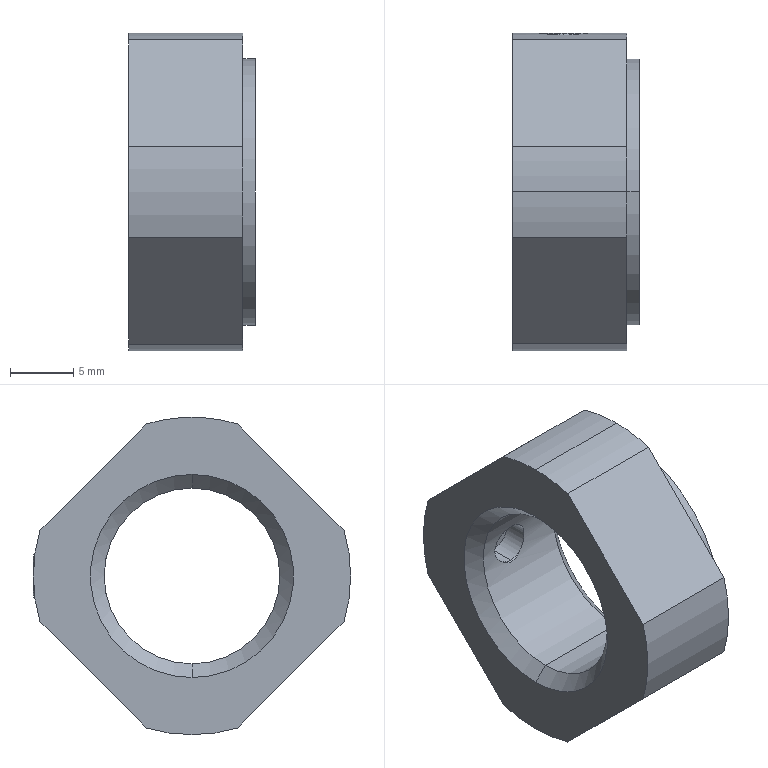Part | STEP file | BNG16 | 2 solids | 48 faces | box 10 x 25 x 25 mm | volume 2769 mm3 | cone 19 | plane 16 | cylinder 13 | commonest cylinder face diameters 25 x5 3.242 x2 4 x2 13.835 x2 21 x2
STEP:
#1=CARTESIAN_POINT('',(8.918,0.,-6.918));
#2=VERTEX_POINT('',#1);
#3=CARTESIAN_POINT('',(8.918,0.,6.918));
#4=VERTEX_POINT('',#3);
#5=CARTESIAN_POINT('',(8.918,0.,0.));
#6=DIRECTION('',(-1.,0.,0.));
#7=DIRECTION('',(0.,0.,1.));
#8=AXIS2_PLACEMENT_3D('',#5,#6,#7);
#9=CIRCLE('',#8,6.918);
#10=EDGE_CURVE('',#2,#4,#9,.T.);
#11=ORIENTED_EDGE('',*,*,#10,.F.);
#12=CARTESIAN_POINT('',(1.083,0.,-6.918));
#13=VERTEX_POINT('',#12);
#14=CARTESIAN_POINT('',(10.,0.,-6.918));
#15=DIRECTION('',(-1.,0.,0.));
#16=VECTOR('',#15,1000.);
#17=LINE('',#14,#16);
#18=EDGE_CURVE('',#2,#13,#17,.T.);
#19=ORIENTED_EDGE('',*,*,#18,.T.);
#20=CARTESIAN_POINT('',(1.083,0.,6.918));
#21=VERTEX_POINT('',#20);
#22=CARTESIAN_POINT('',(1.083,0.,0.));
#23=DIRECTION('',(1.,0.,0.));
#24=DIRECTION('',(0.,0.,1.));
#25=AXIS2_PLACEMENT_3D('',#22,#23,#24);
#26=CIRCLE('',#25,6.918);
#27=EDGE_CURVE('',#21,#13,#26,.T.);
#28=ORIENTED_EDGE('',*,*,#27,.F.);
#29=CARTESIAN_POINT('',(10.,0.,6.918));
#30=DIRECTION('',(-1.,0.,0.));
#31=VECTOR('',#30,1000.);
#32=LINE('',#29,#31);
#33=EDGE_CURVE('',#4,#21,#32,.T.);
#34=ORIENTED_EDGE('',*,*,#33,.F.);
#35=EDGE_LOOP('',(#11,#19,#28,#34));
#36=FACE_OUTER_BOUND('',#35,.T.);
#37=CARTESIAN_POINT('',(10.,0.,0.));
#38=DIRECTION('',(-1.,0.,0.));
#39=DIRECTION('',(0.,0.,1.));
#40=AXIS2_PLACEMENT_3D('',#37,#38,#39);
#41=CYLINDRICAL_SURFACE('',#40,6.918);
#42=ADVANCED_FACE('',(#36),#41,.F.);
#43=ORIENTED_EDGE('',*,*,#27,.T.);
#44=CARTESIAN_POINT('',(0.,0.,-8.));
#45=VERTEX_POINT('',#44);
#46=CARTESIAN_POINT('',(0.,0.,-8.));
#47=DIRECTION('',(-0.7071,0.,-0.7071));
#48=VECTOR('',#47,1000.);
#49=LINE('',#46,#48);
#50=EDGE_CURVE('',#13,#45,#49,.T.);
#51=ORIENTED_EDGE('',*,*,#50,.T.);
#52=CARTESIAN_POINT('',(0.,0.,8.));
#53=VERTEX_POINT('',#52);
#54=CARTESIAN_POINT('',(0.,0.,0.));
#55=DIRECTION('',(1.,0.,0.));
#56=DIRECTION('',(0.,0.,1.));
#57=AXIS2_PLACEMENT_3D('',#54,#55,#56);
#58=CIRCLE('',#57,8.);
#59=EDGE_CURVE('',#53,#45,#58,.T.);
#60=ORIENTED_EDGE('',*,*,#59,.F.);
#61=CARTESIAN_POINT('',(0.,0.,8.));
#62=DIRECTION('',(-0.7071,0.,0.7071));
#63=VECTOR('',#62,1000.);
#64=LINE('',#61,#63);
#65=EDGE_CURVE('',#21,#53,#64,.T.);
#66=ORIENTED_EDGE('',*,*,#65,.F.);
#67=EDGE_LOOP('',(#43,#51,#60,#66));
#68=FACE_OUTER_BOUND('',#67,.T.);
#69=CARTESIAN_POINT('',(0.,0.,0.));
#70=DIRECTION('',(-1.,0.,0.));
#71=DIRECTION('',(0.,0.,1.));
#72=AXIS2_PLACEMENT_3D('',#69,#70,#71);
#73=CONICAL_SURFACE('',#72,8.,0.7854);
#74=ADVANCED_FACE('',(#68),#73,.F.);
#75=CARTESIAN_POINT('',(4.,6.797,-1.621));
#76=VERTEX_POINT('',#75);
#77=CARTESIAN_POINT('',(3.016,6.796,-1.288));
#78=VERTEX_POINT('',#77);
#79=CARTESIAN_POINT('',(4.,6.797,0.));
#80=DIRECTION('',(0.,1.,0.));
#81=DIRECTION('',(0.,0.,1.));
#82=AXIS2_PLACEMENT_3D('',#79,#80,#81);
#83=CIRCLE('',#82,1.621);
#84=EDGE_CURVE('',#76,#78,#83,.T.);
#85=ORIENTED_EDGE('',*,*,#84,.F.);
#86=CARTESIAN_POINT('',(4.,12.121,-1.621));
#87=VERTEX_POINT('',#86);
#88=CARTESIAN_POINT('',(4.,6.418,-1.621));
#89=DIRECTION('',(0.,1.,0.));
#90=VECTOR('',#89,1000.);
#91=LINE('',#88,#90);
#92=EDGE_CURVE('',#76,#87,#91,.T.);
#93=ORIENTED_EDGE('',*,*,#92,.T.);
#94=CARTESIAN_POINT('',(4.,12.121,1.621));
#95=VERTEX_POINT('',#94);
#96=CARTESIAN_POINT('',(4.,12.121,0.));
#97=DIRECTION('',(0.,-1.,0.));
#98=DIRECTION('',(0.,0.,1.));
#99=AXIS2_PLACEMENT_3D('',#96,#97,#98);
#100=CIRCLE('',#99,1.621);
#101=EDGE_CURVE('',#95,#87,#100,.T.);
#102=ORIENTED_EDGE('',*,*,#101,.F.);
#103=CARTESIAN_POINT('',(4.,6.797,1.621));
#104=VERTEX_POINT('',#103);
#105=CARTESIAN_POINT('',(4.,6.418,1.621));
#106=DIRECTION('',(0.,1.,0.));
#107=VECTOR('',#106,1000.);
#108=LINE('',#105,#107);
#109=EDGE_CURVE('',#104,#95,#108,.T.);
#110=ORIENTED_EDGE('',*,*,#109,.F.);
#111=CARTESIAN_POINT('',(3.016,6.797,1.288));
#112=VERTEX_POINT('',#111);
#113=CARTESIAN_POINT('',(4.,6.797,0.));
#114=DIRECTION('',(0.,1.,0.));
#115=DIRECTION('',(0.,0.,1.));
#116=AXIS2_PLACEMENT_3D('',#113,#114,#115);
#117=CIRCLE('',#116,1.621);
#118=EDGE_CURVE('',#112,#104,#117,.T.);
#119=ORIENTED_EDGE('',*,*,#118,.F.);
#120=CARTESIAN_POINT('',(3.016,6.797,1.288));
#121=CARTESIAN_POINT('',(2.917,6.811,1.212));
#122=CARTESIAN_POINT('',(2.828,6.826,1.127));
#123=CARTESIAN_POINT('',(2.671,6.854,0.9367));
#124=CARTESIAN_POINT('',(2.603,6.868,0.8309));
#125=CARTESIAN_POINT('',(2.438,6.903,0.4991));
#126=CARTESIAN_POINT('',(2.379,6.917,0.2501));
#127=CARTESIAN_POINT('',(2.379,6.918,-0.1225));
#128=CARTESIAN_POINT('',(2.393,6.914,-0.2484));
#129=CARTESIAN_POINT('',(2.45,6.901,-0.4896));
#130=CARTESIAN_POINT('',(2.492,6.892,-0.6074));
#131=CARTESIAN_POINT('',(2.602,6.868,-0.8305));
#132=CARTESIAN_POINT('',(2.669,6.855,-0.934));
#133=CARTESIAN_POINT('',(2.827,6.826,-1.125));
#134=CARTESIAN_POINT('',(2.917,6.811,-1.212));
#135=CARTESIAN_POINT('',(3.016,6.796,-1.288));
#136=B_SPLINE_CURVE_WITH_KNOTS('',3,(#120,#121,#122,#123,#124,#125,#126,#127,#128,#129,#130,#131,#132,#133,#134,#135),.UNSPECIFIED.,.F.,.F.,(4,2,2,2,2,2,2,4),(0.,0.0003717,0.0007433,0.001487,0.001858,0.00223,0.002602,0.002973),.UNSPECIFIED.);
#137=EDGE_CURVE('',#112,#78,#136,.T.);
#138=ORIENTED_EDGE('',*,*,#137,.T.);
#139=EDGE_LOOP('',(#85,#93,#102,#110,#119,#138));
#140=FACE_OUTER_BOUND('',#139,.T.);
#141=CARTESIAN_POINT('',(4.,6.418,0.));
#142=DIRECTION('',(0.,1.,0.));
#143=DIRECTION('',(0.,0.,1.));
#144=AXIS2_PLACEMENT_3D('',#141,#142,#143);
#145=CYLINDRICAL_SURFACE('',#144,1.621);
#146=ADVANCED_FACE('',(#140),#145,.F.);
#147=ORIENTED_EDGE('',*,*,#10,.T.);
#148=CARTESIAN_POINT('',(10.,0.,8.));
#149=VERTEX_POINT('',#148);
#150=CARTESIAN_POINT('',(10.,0.,8.));
#151=DIRECTION('',(0.7071,0.,0.7071));
#152=VECTOR('',#151,1000.);
#153=LINE('',#150,#152);
#154=EDGE_CURVE('',#4,#149,#153,.T.);
#155=ORIENTED_EDGE('',*,*,#154,.T.);
#156=CARTESIAN_POINT('',(10.,0.,-8.));
#157=VERTEX_POINT('',#156);
#158=CARTESIAN_POINT('',(10.,0.,0.));
#159=DIRECTION('',(-1.,0.,0.));
#160=DIRECTION('',(0.,0.,-1.));
#161=AXIS2_PLACEMENT_3D('',#158,#159,#160);
#162=CIRCLE('',#161,8.);
#163=EDGE_CURVE('',#157,#149,#162,.T.);
#164=ORIENTED_EDGE('',*,*,#163,.F.);
#165=CARTESIAN_POINT('',(10.,0.,-8.));
#166=DIRECTION('',(0.7071,0.,-0.7071));
#167=VECTOR('',#166,1000.);
#168=LINE('',#165,#167);
#169=EDGE_CURVE('',#2,#157,#168,.T.);
#170=ORIENTED_EDGE('',*,*,#169,.F.);
#171=EDGE_LOOP('',(#147,#155,#164,#170));
#172=FACE_OUTER_BOUND('',#171,.T.);
#173=CARTESIAN_POINT('',(10.,0.,0.));
#174=DIRECTION('',(1.,0.,0.));
#175=DIRECTION('',(0.,0.,-1.));
#176=AXIS2_PLACEMENT_3D('',#173,#174,#175);
#177=CONICAL_SURFACE('',#176,8.,0.7854);
#178=ADVANCED_FACE('',(#172),#177,.F.);
#179=ORIENTED_EDGE('',*,*,#101,.T.);
#180=CARTESIAN_POINT('',(4.,12.361,-1.861));
#181=VERTEX_POINT('',#180);
#182=CARTESIAN_POINT('',(4.,12.504,-2.004));
#183=DIRECTION('',(0.,0.7071,-0.7071));
#184=VECTOR('',#183,1000.);
#185=LINE('',#182,#184);
#186=EDGE_CURVE('',#87,#181,#185,.T.);
#187=ORIENTED_EDGE('',*,*,#186,.T.);
#188=CARTESIAN_POINT('',(4.,12.361,1.861));
#189=VERTEX_POINT('',#188);
#190=CARTESIAN_POINT('',(4.,12.361,1.861));
#191=CARTESIAN_POINT('',(3.748,12.361,1.861));
#192=CARTESIAN_POINT('',(3.493,12.368,1.815));
#193=CARTESIAN_POINT('',(3.022,12.392,1.64));
#194=CARTESIAN_POINT('',(2.8,12.41,1.507));
#195=CARTESIAN_POINT('',(2.427,12.446,1.172));
#196=CARTESIAN_POINT('',(2.271,12.465,0.9655));
#197=CARTESIAN_POINT('',(2.058,12.492,0.51));
#198=CARTESIAN_POINT('',(2.,12.5,0.2533));
#199=CARTESIAN_POINT('',(2.,12.5,-0.1267));
#200=CARTESIAN_POINT('',(2.014,12.498,-0.2518));
#201=CARTESIAN_POINT('',(2.069,12.491,-0.4988));
#202=CARTESIAN_POINT('',(2.11,12.485,-0.6203));
#203=CARTESIAN_POINT('',(2.269,12.465,-0.9631));
#204=CARTESIAN_POINT('',(2.424,12.446,-1.17));
#205=CARTESIAN_POINT('',(2.706,12.419,-1.423));
#206=CARTESIAN_POINT('',(2.809,12.41,-1.498));
#207=CARTESIAN_POINT('',(3.025,12.394,-1.628));
#208=CARTESIAN_POINT('',(3.138,12.386,-1.683));
#209=CARTESIAN_POINT('',(3.495,12.368,-1.816));
#210=CARTESIAN_POINT('',(3.745,12.361,-1.861));
#211=CARTESIAN_POINT('',(4.,12.361,-1.861));
#212=B_SPLINE_CURVE_WITH_KNOTS('',3,(#190,#191,#192,#193,#194,#195,#196,#197,#198,#199,#200,#201,#202,#203,#204,#205,#206,#207,#208,#209,#210,#211),.UNSPECIFIED.,.F.,.F.,(4,2,2,2,2,2,2,2,2,2,4),(0.009167,0.009923,0.01068,0.01143,0.01219,0.01257,0.01294,0.0137,0.01408,0.01445,0.01521),.UNSPECIFIED.);
#213=EDGE_CURVE('',#189,#181,#212,.T.);
#214=ORIENTED_EDGE('',*,*,#213,.F.);
#215=CARTESIAN_POINT('',(4.,12.504,2.004));
#216=DIRECTION('',(0.,0.7071,0.7071));
#217=VECTOR('',#216,1000.);
#218=LINE('',#215,#217);
#219=EDGE_CURVE('',#95,#189,#218,.T.);
#220=ORIENTED_EDGE('',*,*,#219,.F.);
#221=EDGE_LOOP('',(#179,#187,#214,#220));
#222=FACE_OUTER_BOUND('',#221,.T.);
#223=CARTESIAN_POINT('',(4.,12.504,0.));
#224=DIRECTION('',(0.,1.,0.));
#225=DIRECTION('',(0.,0.,1.));
#226=AXIS2_PLACEMENT_3D('',#223,#224,#225);
#227=CONICAL_SURFACE('',#226,2.004,0.7854);
#228=ADVANCED_FACE('',(#222),#227,.F.);
#229=CARTESIAN_POINT('',(9.,-3.58,11.976));
#230=VERTEX_POINT('',#229);
#231=CARTESIAN_POINT('',(9.,0.,12.5));
#232=VERTEX_POINT('',#231);
#233=CARTESIAN_POINT('',(9.,0.,0.));
#234=DIRECTION('',(-1.,0.,0.));
#235=DIRECTION('',(0.,0.,1.));
#236=AXIS2_PLACEMENT_3D('',#233,#234,#235);
#237=CIRCLE('',#236,12.5);
#238=EDGE_CURVE('',#230,#232,#237,.T.);
#239=ORIENTED_EDGE('',*,*,#238,.T.);
#240=CARTESIAN_POINT('',(0.,0.,12.5));
#241=VERTEX_POINT('',#240);
#242=CARTESIAN_POINT('',(10.,0.,12.5));
#243=DIRECTION('',(-1.,0.,0.));
#244=VECTOR('',#243,1000.);
#245=LINE('',#242,#244);
#246=EDGE_CURVE('',#232,#241,#245,.T.);
#247=ORIENTED_EDGE('',*,*,#246,.T.);
#248=CARTESIAN_POINT('',(0.,-3.58,11.976));
#249=VERTEX_POINT('',#248);
#250=CARTESIAN_POINT('',(0.,0.,0.));
#251=DIRECTION('',(-1.,0.,0.));
#252=DIRECTION('',(0.,0.,1.));
#253=AXIS2_PLACEMENT_3D('',#250,#251,#252);
#254=CIRCLE('',#253,12.5);
#255=EDGE_CURVE('',#249,#241,#254,.T.);
#256=ORIENTED_EDGE('',*,*,#255,.F.);
#257=CARTESIAN_POINT('',(10.,-3.58,11.976));
#258=DIRECTION('',(1.,0.,0.));
#259=VECTOR('',#258,1000.);
#260=LINE('',#257,#259);
#261=EDGE_CURVE('',#249,#230,#260,.T.);
#262=ORIENTED_EDGE('',*,*,#261,.T.);
#263=EDGE_LOOP('',(#239,#247,#256,#262));
#264=FACE_OUTER_BOUND('',#263,.T.);
#265=CARTESIAN_POINT('',(10.,0.,0.));
#266=DIRECTION('',(-1.,0.,0.));
#267=DIRECTION('',(0.,0.,1.));
#268=AXIS2_PLACEMENT_3D('',#265,#266,#267);
#269=CYLINDRICAL_SURFACE('',#268,12.5);
#270=ADVANCED_FACE('',(#264),#269,.T.);
#271=CARTESIAN_POINT('',(10.,0.,-10.5));
#272=VERTEX_POINT('',#271);
#273=CARTESIAN_POINT('',(10.,0.,10.5));
#274=VERTEX_POINT('',#273);
#275=CARTESIAN_POINT('',(10.,0.,0.));
#276=DIRECTION('',(1.,0.,0.));
#277=DIRECTION('',(0.,0.,1.));
#278=AXIS2_PLACEMENT_3D('',#275,#276,#277);
#279=CIRCLE('',#278,10.5);
#280=EDGE_CURVE('',#272,#274,#279,.T.);
#281=ORIENTED_EDGE('',*,*,#280,.F.);
#282=CARTESIAN_POINT('',(9.,0.,-10.5));
#283=VERTEX_POINT('',#282);
#284=CARTESIAN_POINT('',(10.,0.,-10.5));
#285=DIRECTION('',(-1.,0.,0.));
#286=VECTOR('',#285,1000.);
#287=LINE('',#284,#286);
#288=EDGE_CURVE('',#272,#283,#287,.T.);
#289=ORIENTED_EDGE('',*,*,#288,.T.);
#290=CARTESIAN_POINT('',(9.,0.,10.5));
#291=VERTEX_POINT('',#290);
#292=CARTESIAN_POINT('',(9.,0.,0.));
#293=DIRECTION('',(1.,0.,0.));
#294=DIRECTION('',(0.,0.,1.));
#295=AXIS2_PLACEMENT_3D('',#292,#293,#294);
#296=CIRCLE('',#295,10.5);
#297=EDGE_CURVE('',#283,#291,#296,.T.);
#298=ORIENTED_EDGE('',*,*,#297,.T.);
#299=CARTESIAN_POINT('',(10.,0.,10.5));
#300=DIRECTION('',(-1.,0.,0.));
#301=VECTOR('',#300,1000.);
#302=LINE('',#299,#301);
#303=EDGE_CURVE('',#274,#291,#302,.T.);
#304=ORIENTED_EDGE('',*,*,#303,.F.);
#305=EDGE_LOOP('',(#281,#289,#298,#304));
#306=FACE_OUTER_BOUND('',#305,.T.);
#307=CARTESIAN_POINT('',(10.,0.,0.));
#308=DIRECTION('',(-1.,0.,0.));
#309=DIRECTION('',(0.,0.,1.));
#310=AXIS2_PLACEMENT_3D('',#307,#308,#309);
#311=CYLINDRICAL_SURFACE('',#310,10.5);
#312=ADVANCED_FACE('',(#306),#311,.T.);
#313=ORIENTED_EDGE('',*,*,#18,.F.);
#314=CARTESIAN_POINT('',(8.918,0.,0.));
#315=DIRECTION('',(-1.,0.,0.));
#316=DIRECTION('',(0.,0.,1.));
#317=AXIS2_PLACEMENT_3D('',#314,#315,#316);
#318=CIRCLE('',#317,6.918);
#319=EDGE_CURVE('',#4,#2,#318,.T.);
#320=ORIENTED_EDGE('',*,*,#319,.F.);
#321=ORIENTED_EDGE('',*,*,#33,.T.);
#322=CARTESIAN_POINT('',(1.083,0.,0.));
#323=DIRECTION('',(1.,0.,0.));
#324=DIRECTION('',(0.,0.,1.));
#325=AXIS2_PLACEMENT_3D('',#322,#323,#324);
#326=CIRCLE('',#325,6.918);
#327=EDGE_CURVE('',#13,#21,#326,.T.);
#328=ORIENTED_EDGE('',*,*,#327,.F.);
#329=EDGE_LOOP('',(#313,#320,#321,#328));
#330=FACE_OUTER_BOUND('',#329,.T.);
#331=CARTESIAN_POINT('',(4.984,6.796,1.288));
#332=VERTEX_POINT('',#331);
#333=CARTESIAN_POINT('',(4.984,6.796,1.288));
#334=CARTESIAN_POINT('',(4.919,6.784,1.353));
#335=CARTESIAN_POINT('',(4.849,6.772,1.412));
#336=CARTESIAN_POINT('',(4.7,6.749,1.517));
#337=CARTESIAN_POINT('',(4.62,6.739,1.563));
#338=CARTESIAN_POINT('',(4.452,6.721,1.638));
#339=CARTESIAN_POINT('',(4.366,6.714,1.667));
#340=CARTESIAN_POINT('',(4.187,6.704,1.706));
#341=CARTESIAN_POINT('',(4.094,6.701,1.716));
#342=CARTESIAN_POINT('',(3.817,6.701,1.717));
#343=CARTESIAN_POINT('',(3.633,6.712,1.676));
#344=CARTESIAN_POINT('',(3.299,6.747,1.527));
#345=CARTESIAN_POINT('',(3.146,6.772,1.419));
#346=CARTESIAN_POINT('',(3.016,6.797,1.288));
#347=B_SPLINE_CURVE_WITH_KNOTS('',3,(#333,#334,#335,#336,#337,#338,#339,#340,#341,#342,#343,#344,#345,#346),.UNSPECIFIED.,.F.,.F.,(4,2,2,2,2,2,4),(0.,0.0002754,0.0005508,0.0008262,0.001102,0.001652,0.002203),.UNSPECIFIED.);
#348=EDGE_CURVE('',#332,#112,#347,.T.);
#349=ORIENTED_EDGE('',*,*,#348,.F.);
#350=CARTESIAN_POINT('',(4.984,6.797,-1.288));
#351=VERTEX_POINT('',#350);
#352=CARTESIAN_POINT('',(4.984,6.797,-1.288));
#353=CARTESIAN_POINT('',(5.083,6.811,-1.212));
#354=CARTESIAN_POINT('',(5.172,6.826,-1.127));
#355=CARTESIAN_POINT('',(5.329,6.854,-0.9367));
#356=CARTESIAN_POINT('',(5.397,6.868,-0.8309));
#357=CARTESIAN_POINT('',(5.562,6.903,-0.4991));
#358=CARTESIAN_POINT('',(5.621,6.917,-0.2501));
#359=CARTESIAN_POINT('',(5.621,6.918,0.1225));
#360=CARTESIAN_POINT('',(5.607,6.914,0.2484));
#361=CARTESIAN_POINT('',(5.55,6.901,0.4896));
#362=CARTESIAN_POINT('',(5.508,6.892,0.6074));
#363=CARTESIAN_POINT('',(5.398,6.868,0.8305));
#364=CARTESIAN_POINT('',(5.331,6.855,0.934));
#365=CARTESIAN_POINT('',(5.173,6.826,1.125));
#366=CARTESIAN_POINT('',(5.083,6.811,1.212));
#367=CARTESIAN_POINT('',(4.984,6.796,1.288));
#368=B_SPLINE_CURVE_WITH_KNOTS('',3,(#352,#353,#354,#355,#356,#357,#358,#359,#360,#361,#362,#363,#364,#365,#366,#367),.UNSPECIFIED.,.F.,.F.,(4,2,2,2,2,2,2,4),(0.,0.0003717,0.0007433,0.001487,0.001858,0.00223,0.002602,0.002973),.UNSPECIFIED.);
#369=EDGE_CURVE('',#351,#332,#368,.T.);
#370=ORIENTED_EDGE('',*,*,#369,.F.);
#371=CARTESIAN_POINT('',(3.016,6.796,-1.288));
#372=CARTESIAN_POINT('',(3.081,6.784,-1.353));
#373=CARTESIAN_POINT('',(3.151,6.772,-1.412));
#374=CARTESIAN_POINT('',(3.3,6.749,-1.517));
#375=CARTESIAN_POINT('',(3.38,6.739,-1.563));
#376=CARTESIAN_POINT('',(3.548,6.721,-1.638));
#377=CARTESIAN_POINT('',(3.634,6.714,-1.667));
#378=CARTESIAN_POINT('',(3.813,6.704,-1.706));
#379=CARTESIAN_POINT('',(3.906,6.701,-1.716));
#380=CARTESIAN_POINT('',(4.183,6.701,-1.717));
#381=CARTESIAN_POINT('',(4.367,6.712,-1.676));
#382=CARTESIAN_POINT('',(4.701,6.747,-1.527));
#383=CARTESIAN_POINT('',(4.854,6.772,-1.419));
#384=CARTESIAN_POINT('',(4.984,6.797,-1.288));
#385=B_SPLINE_CURVE_WITH_KNOTS('',3,(#371,#372,#373,#374,#375,#376,#377,#378,#379,#380,#381,#382,#383,#384),.UNSPECIFIED.,.F.,.F.,(4,2,2,2,2,2,4),(0.,0.0002754,0.0005508,0.0008262,0.001102,0.001652,0.002203),.UNSPECIFIED.);
#386=EDGE_CURVE('',#78,#351,#385,.T.);
#387=ORIENTED_EDGE('',*,*,#386,.F.);
#388=ORIENTED_EDGE('',*,*,#137,.F.);
#389=EDGE_LOOP('',(#349,#370,#387,#388));
#390=FACE_BOUND('',#389,.T.);
#391=CARTESIAN_POINT('',(10.,0.,0.));
#392=DIRECTION('',(-1.,0.,0.));
#393=DIRECTION('',(0.,0.,1.));
#394=AXIS2_PLACEMENT_3D('',#391,#392,#393);
#395=CYLINDRICAL_SURFACE('',#394,6.918);
#396=ADVANCED_FACE('',(#330,#390),#395,.F.);
#397=ORIENTED_EDGE('',*,*,#50,.F.);
#398=ORIENTED_EDGE('',*,*,#327,.T.);
#399=ORIENTED_EDGE('',*,*,#65,.T.);
#400=CARTESIAN_POINT('',(0.,0.,0.));
#401=DIRECTION('',(1.,0.,0.));
#402=DIRECTION('',(0.,0.,1.));
#403=AXIS2_PLACEMENT_3D('',#400,#401,#402);
#404=CIRCLE('',#403,8.);
#405=EDGE_CURVE('',#45,#53,#404,.T.);
#406=ORIENTED_EDGE('',*,*,#405,.F.);
#407=EDGE_LOOP('',(#397,#398,#399,#406));
#408=FACE_OUTER_BOUND('',#407,.T.);
#409=CARTESIAN_POINT('',(0.,0.,0.));
#410=DIRECTION('',(-1.,0.,0.));
#411=DIRECTION('',(0.,0.,1.));
#412=AXIS2_PLACEMENT_3D('',#409,#410,#411);
#413=CONICAL_SURFACE('',#412,8.,0.7854);
#414=ADVANCED_FACE('',(#408),#413,.F.);
#415=ORIENTED_EDGE('',*,*,#92,.F.);
#416=CARTESIAN_POINT('',(4.,6.797,0.));
#417=DIRECTION('',(0.,1.,0.));
#418=DIRECTION('',(0.,0.,1.));
#419=AXIS2_PLACEMENT_3D('',#416,#417,#418);
#420=CIRCLE('',#419,1.621);
#421=EDGE_CURVE('',#351,#76,#420,.T.);
#422=ORIENTED_EDGE('',*,*,#421,.F.);
#423=ORIENTED_EDGE('',*,*,#369,.T.);
#424=CARTESIAN_POINT('',(4.,6.797,0.));
#425=DIRECTION('',(0.,1.,0.));
#426=DIRECTION('',(0.,0.,1.));
#427=AXIS2_PLACEMENT_3D('',#424,#425,#426);
#428=CIRCLE('',#427,1.621);
#429=EDGE_CURVE('',#104,#332,#428,.T.);
#430=ORIENTED_EDGE('',*,*,#429,.F.);
#431=ORIENTED_EDGE('',*,*,#109,.T.);
#432=CARTESIAN_POINT('',(4.,12.121,0.));
#433=DIRECTION('',(0.,-1.,0.));
#434=DIRECTION('',(0.,0.,1.));
#435=AXIS2_PLACEMENT_3D('',#432,#433,#434);
#436=CIRCLE('',#435,1.621);
#437=EDGE_CURVE('',#87,#95,#436,.T.);
#438=ORIENTED_EDGE('',*,*,#437,.F.);
#439=EDGE_LOOP('',(#415,#422,#423,#430,#431,#438));
#440=FACE_OUTER_BOUND('',#439,.T.);
#441=CARTESIAN_POINT('',(4.,6.418,0.));
#442=DIRECTION('',(0.,1.,0.));
#443=DIRECTION('',(0.,0.,1.));
#444=AXIS2_PLACEMENT_3D('',#441,#442,#443);
#445=CYLINDRICAL_SURFACE('',#444,1.621);
#446=ADVANCED_FACE('',(#440),#445,.F.);
#447=ORIENTED_EDGE('',*,*,#348,.T.);
#448=ORIENTED_EDGE('',*,*,#118,.T.);
#449=ORIENTED_EDGE('',*,*,#429,.T.);
#450=EDGE_LOOP('',(#447,#448,#449));
#451=FACE_OUTER_BOUND('',#450,.T.);
#452=CARTESIAN_POINT('',(4.,6.701,0.));
#453=DIRECTION('',(0.,-1.,0.));
#454=DIRECTION('',(0.,0.,-1.));
#455=AXIS2_PLACEMENT_3D('',#452,#453,#454);
#456=CONICAL_SURFACE('',#455,1.717,0.7854);
#457=ADVANCED_FACE('',(#451),#456,.F.);
#458=ORIENTED_EDGE('',*,*,#386,.T.);
#459=ORIENTED_EDGE('',*,*,#421,.T.);
#460=ORIENTED_EDGE('',*,*,#84,.T.);
#461=EDGE_LOOP('',(#458,#459,#460));
#462=FACE_OUTER_BOUND('',#461,.T.);
#463=CARTESIAN_POINT('',(4.,6.701,0.));
#464=DIRECTION('',(0.,-1.,0.));
#465=DIRECTION('',(1.,0.,0.));
#466=AXIS2_PLACEMENT_3D('',#463,#464,#465);
#467=CONICAL_SURFACE('',#466,1.717,0.7854);
#468=ADVANCED_FACE('',(#462),#467,.F.);
#469=ORIENTED_EDGE('',*,*,#154,.F.);
#470=ORIENTED_EDGE('',*,*,#319,.T.);
#471=ORIENTED_EDGE('',*,*,#169,.T.);
#472=CARTESIAN_POINT('',(10.,0.,0.));
#473=DIRECTION('',(-1.,0.,0.));
#474=DIRECTION('',(0.,0.,-1.));
#475=AXIS2_PLACEMENT_3D('',#472,#473,#474);
#476=CIRCLE('',#475,8.);
#477=EDGE_CURVE('',#149,#157,#476,.T.);
#478=ORIENTED_EDGE('',*,*,#477,.F.);
#479=EDGE_LOOP('',(#469,#470,#471,#478));
#480=FACE_OUTER_BOUND('',#479,.T.);
#481=CARTESIAN_POINT('',(10.,0.,0.));
#482=DIRECTION('',(1.,0.,0.));
#483=DIRECTION('',(0.,0.,-1.));
#484=AXIS2_PLACEMENT_3D('',#481,#482,#483);
#485=CONICAL_SURFACE('',#484,8.,0.7854);
#486=ADVANCED_FACE('',(#480),#485,.F.);
#487=CARTESIAN_POINT('',(0.,-11.976,3.58));
#488=VERTEX_POINT('',#487);
#489=CARTESIAN_POINT('',(0.,-11.976,3.58));
#490=DIRECTION('',(0.,0.7071,0.7071));
#491=VECTOR('',#490,1000.);
#492=LINE('',#489,#491);
#493=EDGE_CURVE('',#488,#249,#492,.T.);
#494=ORIENTED_EDGE('',*,*,#493,.T.);
#495=ORIENTED_EDGE('',*,*,#255,.T.);
#496=CARTESIAN_POINT('',(0.,3.58,11.976));
#497=VERTEX_POINT('',#496);
#498=CARTESIAN_POINT('',(0.,0.,0.));
#499=DIRECTION('',(-1.,0.,0.));
#500=DIRECTION('',(0.,0.,1.));
#501=AXIS2_PLACEMENT_3D('',#498,#499,#500);
#502=CIRCLE('',#501,12.5);
#503=EDGE_CURVE('',#241,#497,#502,.T.);
#504=ORIENTED_EDGE('',*,*,#503,.T.);
#505=CARTESIAN_POINT('',(0.,11.976,3.58));
#506=VERTEX_POINT('',#505);
#507=CARTESIAN_POINT('',(0.,3.58,11.976));
#508=DIRECTION('',(0.,0.7071,-0.7071));
#509=VECTOR('',#508,1000.);
#510=LINE('',#507,#509);
#511=EDGE_CURVE('',#497,#506,#510,.T.);
#512=ORIENTED_EDGE('',*,*,#511,.T.);
#513=CARTESIAN_POINT('',(0.,11.976,-3.58));
#514=VERTEX_POINT('',#513);
#515=CARTESIAN_POINT('',(0.,0.,0.));
#516=DIRECTION('',(-1.,0.,0.));
#517=DIRECTION('',(0.,0.,1.));
#518=AXIS2_PLACEMENT_3D('',#515,#516,#517);
#519=CIRCLE('',#518,12.5);
#520=EDGE_CURVE('',#506,#514,#519,.T.);
#521=ORIENTED_EDGE('',*,*,#520,.T.);
#522=CARTESIAN_POINT('',(0.,3.58,-11.976));
#523=VERTEX_POINT('',#522);
#524=CARTESIAN_POINT('',(0.,11.976,-3.58));
#525=DIRECTION('',(0.,-0.7071,-0.7071));
#526=VECTOR('',#525,1000.);
#527=LINE('',#524,#526);
#528=EDGE_CURVE('',#514,#523,#527,.T.);
#529=ORIENTED_EDGE('',*,*,#528,.T.);
#530=CARTESIAN_POINT('',(0.,-3.58,-11.976));
#531=VERTEX_POINT('',#530);
#532=CARTESIAN_POINT('',(0.,0.,0.));
#533=DIRECTION('',(-1.,0.,0.));
#534=DIRECTION('',(0.,0.,1.));
#535=AXIS2_PLACEMENT_3D('',#532,#533,#534);
#536=CIRCLE('',#535,12.5);
#537=EDGE_CURVE('',#523,#531,#536,.T.);
#538=ORIENTED_EDGE('',*,*,#537,.T.);
#539=CARTESIAN_POINT('',(0.,-11.976,-3.58));
#540=VERTEX_POINT('',#539);
#541=CARTESIAN_POINT('',(0.,-3.58,-11.976));
#542=DIRECTION('',(0.,-0.7071,0.7071));
#543=VECTOR('',#542,1000.);
#544=LINE('',#541,#543);
#545=EDGE_CURVE('',#531,#540,#544,.T.);
#546=ORIENTED_EDGE('',*,*,#545,.T.);
#547=CARTESIAN_POINT('',(0.,0.,0.));
#548=DIRECTION('',(-1.,0.,0.));
#549=DIRECTION('',(0.,0.,1.));
#550=AXIS2_PLACEMENT_3D('',#547,#548,#549);
#551=CIRCLE('',#550,12.5);
#552=EDGE_CURVE('',#540,#488,#551,.T.);
#553=ORIENTED_EDGE('',*,*,#552,.T.);
#554=EDGE_LOOP('',(#494,#495,#504,#512,#521,#529,#538,#546,#553));
#555=FACE_OUTER_BOUND('',#554,.T.);
#556=ORIENTED_EDGE('',*,*,#59,.T.);
#557=ORIENTED_EDGE('',*,*,#405,.T.);
#558=EDGE_LOOP('',(#556,#557));
#559=FACE_BOUND('',#558,.T.);
#560=CARTESIAN_POINT('',(0.,12.5,0.));
#561=DIRECTION('',(-1.,0.,0.));
#562=DIRECTION('',(0.,0.,1.));
#563=AXIS2_PLACEMENT_3D('',#560,#561,#562);
#564=PLANE('',#563);
#565=ADVANCED_FACE('',(#555,#559),#564,.T.);
#566=ORIENTED_EDGE('',*,*,#186,.F.);
#567=ORIENTED_EDGE('',*,*,#437,.T.);
#568=ORIENTED_EDGE('',*,*,#219,.T.);
#569=CARTESIAN_POINT('',(4.,12.361,-1.861));
#570=CARTESIAN_POINT('',(4.255,12.361,-1.861));
#571=CARTESIAN_POINT('',(4.505,12.368,-1.816));
#572=CARTESIAN_POINT('',(4.861,12.386,-1.683));
#573=CARTESIAN_POINT('',(4.974,12.394,-1.629));
#574=CARTESIAN_POINT('',(5.19,12.41,-1.499));
#575=CARTESIAN_POINT('',(5.293,12.419,-1.424));
#576=CARTESIAN_POINT('',(5.481,12.437,-1.255));
#577=CARTESIAN_POINT('',(5.566,12.446,-1.163));
#578=CARTESIAN_POINT('',(5.716,12.463,-0.9615));
#579=CARTESIAN_POINT('',(5.783,12.472,-0.8511));
#580=CARTESIAN_POINT('',(5.889,12.485,-0.6228));
#581=CARTESIAN_POINT('',(5.93,12.49,-0.504));
#582=CARTESIAN_POINT('',(5.985,12.498,-0.2565));
#583=CARTESIAN_POINT('',(6.,12.5,-0.1291));
#584=CARTESIAN_POINT('',(6.,12.5,0.1228));
#585=CARTESIAN_POINT('',(5.986,12.498,0.25));
#586=CARTESIAN_POINT('',(5.932,12.491,0.498));
#587=CARTESIAN_POINT('',(5.891,12.485,0.6174));
#588=CARTESIAN_POINT('',(5.785,12.472,0.8472));
#589=CARTESIAN_POINT('',(5.719,12.464,0.9573));
#590=CARTESIAN_POINT('',(5.569,12.447,1.159));
#591=CARTESIAN_POINT('',(5.483,12.437,1.253));
#592=CARTESIAN_POINT('',(5.294,12.419,1.423));
#593=CARTESIAN_POINT('',(5.193,12.41,1.497));
#594=CARTESIAN_POINT('',(4.977,12.394,1.627));
#595=CARTESIAN_POINT('',(4.861,12.386,1.683));
#596=CARTESIAN_POINT('',(4.624,12.374,1.771));
#597=CARTESIAN_POINT('',(4.503,12.369,1.805));
#598=CARTESIAN_POINT('',(4.254,12.362,1.849));
#599=CARTESIAN_POINT('',(4.126,12.361,1.861));
#600=CARTESIAN_POINT('',(4.,12.361,1.861));
#601=B_SPLINE_CURVE_WITH_KNOTS('',3,(#569,#570,#571,#572,#573,#574,#575,#576,#577,#578,#579,#580,#581,#582,#583,#584,#585,#586,#587,#588,#589,#590,#591,#592,#593,#594,#595,#596,#597,#598,#599,#600),.UNSPECIFIED.,.F.,.F.,(4,2,2,2,2,2,2,2,2,2,2,2,2,2,2,4),(0.003125,0.00388,0.004258,0.004635,0.005013,0.005391,0.005768,0.006146,0.006524,0.006901,0.007279,0.007657,0.008034,0.008412,0.00879,0.009167),.UNSPECIFIED.);
#602=EDGE_CURVE('',#181,#189,#601,.T.);
#603=ORIENTED_EDGE('',*,*,#602,.F.);
#604=EDGE_LOOP('',(#566,#567,#568,#603));
#605=FACE_OUTER_BOUND('',#604,.T.);
#606=CARTESIAN_POINT('',(4.,12.504,0.));
#607=DIRECTION('',(0.,1.,0.));
#608=DIRECTION('',(0.,0.,1.));
#609=AXIS2_PLACEMENT_3D('',#606,#607,#608);
#610=CONICAL_SURFACE('',#609,2.004,0.7854);
#611=ADVANCED_FACE('',(#605),#610,.F.);
#612=ORIENTED_EDGE('',*,*,#163,.T.);
#613=ORIENTED_EDGE('',*,*,#477,.T.);
#614=EDGE_LOOP('',(#612,#613));
#615=FACE_BOUND('',#614,.T.);
#616=CARTESIAN_POINT('',(10.,0.,0.));
#617=DIRECTION('',(1.,0.,0.));
#618=DIRECTION('',(0.,0.,1.));
#619=AXIS2_PLACEMENT_3D('',#616,#617,#618);
#620=CIRCLE('',#619,10.5);
#621=EDGE_CURVE('',#274,#272,#620,.T.);
#622=ORIENTED_EDGE('',*,*,#621,.T.);
#623=ORIENTED_EDGE('',*,*,#280,.T.);
#624=EDGE_LOOP('',(#622,#623));
#625=FACE_OUTER_BOUND('',#624,.T.);
#626=CARTESIAN_POINT('',(10.,8.,0.));
#627=DIRECTION('',(1.,0.,0.));
#628=DIRECTION('',(0.,0.,-1.));
#629=AXIS2_PLACEMENT_3D('',#626,#627,#628);
#630=PLANE('',#629);
#631=ADVANCED_FACE('',(#615,#625),#630,.T.);
#632=ORIENTED_EDGE('',*,*,#246,.F.);
#633=CARTESIAN_POINT('',(9.,3.58,11.976));
#634=VERTEX_POINT('',#633);
#635=CARTESIAN_POINT('',(9.,0.,0.));
#636=DIRECTION('',(-1.,0.,0.));
#637=DIRECTION('',(0.,0.,1.));
#638=AXIS2_PLACEMENT_3D('',#635,#636,#637);
#639=CIRCLE('',#638,12.5);
#640=EDGE_CURVE('',#232,#634,#639,.T.);
#641=ORIENTED_EDGE('',*,*,#640,.T.);
#642=CARTESIAN_POINT('',(10.,3.58,11.976));
#643=DIRECTION('',(-1.,0.,0.));
#644=VECTOR('',#643,1000.);
#645=LINE('',#642,#644);
#646=EDGE_CURVE('',#634,#497,#645,.T.);
#647=ORIENTED_EDGE('',*,*,#646,.T.);
#648=ORIENTED_EDGE('',*,*,#503,.F.);
#649=EDGE_LOOP('',(#632,#641,#647,#648));
#650=FACE_OUTER_BOUND('',#649,.T.);
#651=CARTESIAN_POINT('',(10.,0.,0.));
#652=DIRECTION('',(-1.,0.,0.));
#653=DIRECTION('',(0.,0.,1.));
#654=AXIS2_PLACEMENT_3D('',#651,#652,#653);
#655=CYLINDRICAL_SURFACE('',#654,12.5);
#656=ADVANCED_FACE('',(#650),#655,.T.);
#657=ORIENTED_EDGE('',*,*,#493,.F.);
#658=CARTESIAN_POINT('',(9.,-11.976,3.58));
#659=VERTEX_POINT('',#658);
#660=CARTESIAN_POINT('',(10.,-11.976,3.58));
#661=DIRECTION('',(-1.,0.,0.));
#662=VECTOR('',#661,1000.);
#663=LINE('',#660,#662);
#664=EDGE_CURVE('',#659,#488,#663,.T.);
#665=ORIENTED_EDGE('',*,*,#664,.F.);
#666=CARTESIAN_POINT('',(9.,0.,15.556));
#667=DIRECTION('',(0.,-0.7071,-0.7071));
#668=VECTOR('',#667,1000.);
#669=LINE('',#666,#668);
#670=EDGE_CURVE('',#230,#659,#669,.T.);
#671=ORIENTED_EDGE('',*,*,#670,.F.);
#672=ORIENTED_EDGE('',*,*,#261,.F.);
#673=EDGE_LOOP('',(#657,#665,#671,#672));
#674=FACE_OUTER_BOUND('',#673,.T.);
#675=CARTESIAN_POINT('',(10.,0.,15.556));
#676=DIRECTION('',(0.,0.7071,-0.7071));
#677=DIRECTION('',(0.,0.7071,0.7071));
#678=AXIS2_PLACEMENT_3D('',#675,#676,#677);
#679=PLANE('',#678);
#680=ADVANCED_FACE('',(#674),#679,.F.);
#681=ORIENTED_EDGE('',*,*,#664,.T.);
#682=ORIENTED_EDGE('',*,*,#552,.F.);
#683=CARTESIAN_POINT('',(9.,-11.976,-3.58));
#684=VERTEX_POINT('',#683);
#685=CARTESIAN_POINT('',(10.,-11.976,-3.58));
#686=DIRECTION('',(1.,0.,0.));
#687=VECTOR('',#686,1000.);
#688=LINE('',#685,#687);
#689=EDGE_CURVE('',#540,#684,#688,.T.);
#690=ORIENTED_EDGE('',*,*,#689,.T.);
#691=CARTESIAN_POINT('',(9.,0.,0.));
#692=DIRECTION('',(-1.,0.,0.));
#693=DIRECTION('',(0.,0.,1.));
#694=AXIS2_PLACEMENT_3D('',#691,#692,#693);
#695=CIRCLE('',#694,12.5);
#696=EDGE_CURVE('',#684,#659,#695,.T.);
#697=ORIENTED_EDGE('',*,*,#696,.T.);
#698=EDGE_LOOP('',(#681,#682,#690,#697));
#699=FACE_OUTER_BOUND('',#698,.T.);
#700=CARTESIAN_POINT('',(10.,0.,0.));
#701=DIRECTION('',(-1.,0.,0.));
#702=DIRECTION('',(0.,0.,1.));
#703=AXIS2_PLACEMENT_3D('',#700,#701,#702);
#704=CYLINDRICAL_SURFACE('',#703,12.5);
#705=ADVANCED_FACE('',(#699),#704,.T.);
#706=ORIENTED_EDGE('',*,*,#545,.F.);
#707=CARTESIAN_POINT('',(9.,-3.58,-11.976));
#708=VERTEX_POINT('',#707);
#709=CARTESIAN_POINT('',(10.,-3.58,-11.976));
#710=DIRECTION('',(-1.,0.,0.));
#711=VECTOR('',#710,1000.);
#712=LINE('',#709,#711);
#713=EDGE_CURVE('',#708,#531,#712,.T.);
#714=ORIENTED_EDGE('',*,*,#713,.F.);
#715=CARTESIAN_POINT('',(9.,-15.556,0.));
#716=DIRECTION('',(0.,0.7071,-0.7071));
#717=VECTOR('',#716,1000.);
#718=LINE('',#715,#717);
#719=EDGE_CURVE('',#684,#708,#718,.T.);
#720=ORIENTED_EDGE('',*,*,#719,.F.);
#721=ORIENTED_EDGE('',*,*,#689,.F.);
#722=EDGE_LOOP('',(#706,#714,#720,#721));
#723=FACE_OUTER_BOUND('',#722,.T.);
#724=CARTESIAN_POINT('',(10.,-15.556,0.));
#725=DIRECTION('',(0.,0.7071,0.7071));
#726=DIRECTION('',(0.,-0.7071,0.7071));
#727=AXIS2_PLACEMENT_3D('',#724,#725,#726);
#728=PLANE('',#727);
#729=ADVANCED_FACE('',(#723),#728,.F.);
#730=ORIENTED_EDGE('',*,*,#713,.T.);
#731=ORIENTED_EDGE('',*,*,#537,.F.);
#732=CARTESIAN_POINT('',(9.,3.58,-11.976));
#733=VERTEX_POINT('',#732);
#734=CARTESIAN_POINT('',(10.,3.58,-11.976));
#735=DIRECTION('',(1.,0.,0.));
#736=VECTOR('',#735,1000.);
#737=LINE('',#734,#736);
#738=EDGE_CURVE('',#523,#733,#737,.T.);
#739=ORIENTED_EDGE('',*,*,#738,.T.);
#740=CARTESIAN_POINT('',(9.,0.,0.));
#741=DIRECTION('',(-1.,0.,0.));
#742=DIRECTION('',(0.,0.,1.));
#743=AXIS2_PLACEMENT_3D('',#740,#741,#742);
#744=CIRCLE('',#743,12.5);
#745=EDGE_CURVE('',#733,#708,#744,.T.);
#746=ORIENTED_EDGE('',*,*,#745,.T.);
#747=EDGE_LOOP('',(#730,#731,#739,#746));
#748=FACE_OUTER_BOUND('',#747,.T.);
#749=CARTESIAN_POINT('',(10.,0.,0.));
#750=DIRECTION('',(-1.,0.,0.));
#751=DIRECTION('',(0.,0.,1.));
#752=AXIS2_PLACEMENT_3D('',#749,#750,#751);
#753=CYLINDRICAL_SURFACE('',#752,12.5);
#754=ADVANCED_FACE('',(#748),#753,.T.);
#755=ORIENTED_EDGE('',*,*,#528,.F.);
#756=CARTESIAN_POINT('',(9.,11.976,-3.58));
#757=VERTEX_POINT('',#756);
#758=CARTESIAN_POINT('',(10.,11.976,-3.58));
#759=DIRECTION('',(-1.,0.,0.));
#760=VECTOR('',#759,1000.);
#761=LINE('',#758,#760);
#762=EDGE_CURVE('',#757,#514,#761,.T.);
#763=ORIENTED_EDGE('',*,*,#762,.F.);
#764=CARTESIAN_POINT('',(9.,0.,-15.556));
#765=DIRECTION('',(0.,0.7071,0.7071));
#766=VECTOR('',#765,1000.);
#767=LINE('',#764,#766);
#768=EDGE_CURVE('',#733,#757,#767,.T.);
#769=ORIENTED_EDGE('',*,*,#768,.F.);
#770=ORIENTED_EDGE('',*,*,#738,.F.);
#771=EDGE_LOOP('',(#755,#763,#769,#770));
#772=FACE_OUTER_BOUND('',#771,.T.);
#773=CARTESIAN_POINT('',(10.,0.,-15.556));
#774=DIRECTION('',(0.,-0.7071,0.7071));
#775=DIRECTION('',(0.,-0.7071,-0.7071));
#776=AXIS2_PLACEMENT_3D('',#773,#774,#775);
#777=PLANE('',#776);
#778=ADVANCED_FACE('',(#772),#777,.F.);
#779=ORIENTED_EDGE('',*,*,#213,.T.);
#780=ORIENTED_EDGE('',*,*,#602,.T.);
#781=EDGE_LOOP('',(#779,#780));
#782=FACE_BOUND('',#781,.T.);
#783=CARTESIAN_POINT('',(9.,11.976,3.58));
#784=VERTEX_POINT('',#783);
#785=CARTESIAN_POINT('',(10.,11.976,3.58));
#786=DIRECTION('',(1.,0.,0.));
#787=VECTOR('',#786,1000.);
#788=LINE('',#785,#787);
#789=EDGE_CURVE('',#506,#784,#788,.T.);
#790=ORIENTED_EDGE('',*,*,#789,.T.);
#791=CARTESIAN_POINT('',(9.,0.,0.));
#792=DIRECTION('',(-1.,0.,0.));
#793=DIRECTION('',(0.,0.,1.));
#794=AXIS2_PLACEMENT_3D('',#791,#792,#793);
#795=CIRCLE('',#794,12.5);
#796=EDGE_CURVE('',#784,#757,#795,.T.);
#797=ORIENTED_EDGE('',*,*,#796,.T.);
#798=ORIENTED_EDGE('',*,*,#762,.T.);
#799=ORIENTED_EDGE('',*,*,#520,.F.);
#800=EDGE_LOOP('',(#790,#797,#798,#799));
#801=FACE_OUTER_BOUND('',#800,.T.);
#802=CARTESIAN_POINT('',(10.,0.,0.));
#803=DIRECTION('',(-1.,0.,0.));
#804=DIRECTION('',(0.,0.,1.));
#805=AXIS2_PLACEMENT_3D('',#802,#803,#804);
#806=CYLINDRICAL_SURFACE('',#805,12.5);
#807=ADVANCED_FACE('',(#782,#801),#806,.T.);
#808=ORIENTED_EDGE('',*,*,#511,.F.);
#809=ORIENTED_EDGE('',*,*,#646,.F.);
#810=CARTESIAN_POINT('',(9.,15.556,0.));
#811=DIRECTION('',(0.,-0.7071,0.7071));
#812=VECTOR('',#811,1000.);
#813=LINE('',#810,#812);
#814=EDGE_CURVE('',#784,#634,#813,.T.);
#815=ORIENTED_EDGE('',*,*,#814,.F.);
#816=ORIENTED_EDGE('',*,*,#789,.F.);
#817=EDGE_LOOP('',(#808,#809,#815,#816));
#818=FACE_OUTER_BOUND('',#817,.T.);
#819=CARTESIAN_POINT('',(10.,15.556,0.));
#820=DIRECTION('',(0.,-0.7071,-0.7071));
#821=DIRECTION('',(0.,0.7071,-0.7071));
#822=AXIS2_PLACEMENT_3D('',#819,#820,#821);
#823=PLANE('',#822);
#824=ADVANCED_FACE('',(#818),#823,.F.);
#825=ORIENTED_EDGE('',*,*,#288,.F.);
#826=ORIENTED_EDGE('',*,*,#621,.F.);
#827=ORIENTED_EDGE('',*,*,#303,.T.);
#828=CARTESIAN_POINT('',(9.,0.,0.));
#829=DIRECTION('',(1.,0.,0.));
#830=DIRECTION('',(0.,0.,1.));
#831=AXIS2_PLACEMENT_3D('',#828,#829,#830);
#832=CIRCLE('',#831,10.5);
#833=EDGE_CURVE('',#291,#283,#832,.T.);
#834=ORIENTED_EDGE('',*,*,#833,.T.);
#835=EDGE_LOOP('',(#825,#826,#827,#834));
#836=FACE_OUTER_BOUND('',#835,.T.);
#837=CARTESIAN_POINT('',(10.,0.,0.));
#838=DIRECTION('',(-1.,0.,0.));
#839=DIRECTION('',(0.,0.,1.));
#840=AXIS2_PLACEMENT_3D('',#837,#838,#839);
#841=CYLINDRICAL_SURFACE('',#840,10.5);
#842=ADVANCED_FACE('',(#836),#841,.T.);
#843=ORIENTED_EDGE('',*,*,#833,.F.);
#844=ORIENTED_EDGE('',*,*,#297,.F.);
#845=EDGE_LOOP('',(#843,#844));
#846=FACE_BOUND('',#845,.T.);
#847=ORIENTED_EDGE('',*,*,#719,.T.);
#848=ORIENTED_EDGE('',*,*,#745,.F.);
#849=ORIENTED_EDGE('',*,*,#768,.T.);
#850=ORIENTED_EDGE('',*,*,#796,.F.);
#851=ORIENTED_EDGE('',*,*,#814,.T.);
#852=ORIENTED_EDGE('',*,*,#640,.F.);
#853=ORIENTED_EDGE('',*,*,#238,.F.);
#854=ORIENTED_EDGE('',*,*,#670,.T.);
#855=ORIENTED_EDGE('',*,*,#696,.F.);
#856=EDGE_LOOP('',(#847,#848,#849,#850,#851,#852,#853,#854,#855));
#857=FACE_OUTER_BOUND('',#856,.T.);
#858=CARTESIAN_POINT('',(9.,10.5,0.));
#859=DIRECTION('',(1.,0.,0.));
#860=DIRECTION('',(0.,0.,-1.));
#861=AXIS2_PLACEMENT_3D('',#858,#859,#860);
#862=PLANE('',#861);
#863=ADVANCED_FACE('',(#846,#857),#862,.T.);
#864=CLOSED_SHELL('',(#42,#74,#146,#178,#228,#270,#312,#396,#414,#446,#457,#468,#486,#565,#611,#631,#656,#680,#705,#729,#754,#778,#807,#824,#842,#863));
#865=MANIFOLD_SOLID_BREP('',#864);
#866=CARTESIAN_POINT('',(4.,12.252,2.));
#867=VERTEX_POINT('',#866);
#868=CARTESIAN_POINT('',(4.,12.252,-2.));
#869=VERTEX_POINT('',#868);
#870=CARTESIAN_POINT('',(4.,12.252,0.));
#871=DIRECTION('',(0.,-1.,0.));
#872=DIRECTION('',(0.,0.,1.));
#873=AXIS2_PLACEMENT_3D('',#870,#871,#872);
#874=CIRCLE('',#873,2.);
#875=EDGE_CURVE('',#867,#869,#874,.T.);
#876=ORIENTED_EDGE('',*,*,#875,.T.);
#877=CARTESIAN_POINT('',(4.,9.25,-2.));
#878=VERTEX_POINT('',#877);
#879=CARTESIAN_POINT('',(4.,11.833,-2.));
#880=DIRECTION('',(0.,-1.,0.));
#881=VECTOR('',#880,1000.);
#882=LINE('',#879,#881);
#883=EDGE_CURVE('',#869,#878,#882,.T.);
#884=ORIENTED_EDGE('',*,*,#883,.T.);
#885=CARTESIAN_POINT('',(2.,9.25,0.));
#886=VERTEX_POINT('',#885);
#887=CARTESIAN_POINT('',(4.,9.25,0.));
#888=DIRECTION('',(0.,1.,0.));
#889=DIRECTION('',(0.,0.,1.));
#890=AXIS2_PLACEMENT_3D('',#887,#888,#889);
#891=CIRCLE('',#890,2.);
#892=EDGE_CURVE('',#878,#886,#891,.T.);
#893=ORIENTED_EDGE('',*,*,#892,.T.);
#894=CARTESIAN_POINT('',(4.,9.25,2.));
#895=VERTEX_POINT('',#894);
#896=CARTESIAN_POINT('',(4.,9.25,0.));
#897=DIRECTION('',(0.,1.,0.));
#898=DIRECTION('',(0.,0.,1.));
#899=AXIS2_PLACEMENT_3D('',#896,#897,#898);
#900=CIRCLE('',#899,2.);
#901=EDGE_CURVE('',#886,#895,#900,.T.);
#902=ORIENTED_EDGE('',*,*,#901,.T.);
#903=CARTESIAN_POINT('',(4.,11.833,2.));
#904=DIRECTION('',(0.,-1.,0.));
#905=VECTOR('',#904,1000.);
#906=LINE('',#903,#905);
#907=EDGE_CURVE('',#867,#895,#906,.T.);
#908=ORIENTED_EDGE('',*,*,#907,.F.);
#909=EDGE_LOOP('',(#876,#884,#893,#902,#908));
#910=FACE_OUTER_BOUND('',#909,.T.);
#911=CARTESIAN_POINT('',(4.,11.833,0.));
#912=DIRECTION('',(0.,-1.,0.));
#913=DIRECTION('',(0.,0.,1.));
#914=AXIS2_PLACEMENT_3D('',#911,#912,#913);
#915=CYLINDRICAL_SURFACE('',#914,2.);
#916=ADVANCED_FACE('',(#910),#915,.T.);
#917=CARTESIAN_POINT('',(2.75,8.5,0.));
#918=VERTEX_POINT('',#917);
#919=CARTESIAN_POINT('',(5.25,8.5,0.));
#920=VERTEX_POINT('',#919);
#921=CARTESIAN_POINT('',(4.,8.5,0.));
#922=DIRECTION('',(0.,1.,0.));
#923=DIRECTION('',(-1.,0.,0.));
#924=AXIS2_PLACEMENT_3D('',#921,#922,#923);
#925=CIRCLE('',#924,1.25);
#926=EDGE_CURVE('',#918,#920,#925,.T.);
#927=ORIENTED_EDGE('',*,*,#926,.T.);
#928=CARTESIAN_POINT('',(6.,9.25,0.));
#929=VERTEX_POINT('',#928);
#930=CARTESIAN_POINT('',(6.,9.25,0.));
#931=DIRECTION('',(0.7071,0.7071,0.));
#932=VECTOR('',#931,1000.);
#933=LINE('',#930,#932);
#934=EDGE_CURVE('',#920,#929,#933,.T.);
#935=ORIENTED_EDGE('',*,*,#934,.T.);
#936=CARTESIAN_POINT('',(4.,9.25,0.));
#937=DIRECTION('',(0.,1.,0.));
#938=DIRECTION('',(0.,0.,1.));
#939=AXIS2_PLACEMENT_3D('',#936,#937,#938);
#940=CIRCLE('',#939,2.);
#941=EDGE_CURVE('',#895,#929,#940,.T.);
#942=ORIENTED_EDGE('',*,*,#941,.F.);
#943=ORIENTED_EDGE('',*,*,#901,.F.);
#944=CARTESIAN_POINT('',(2.,9.25,0.));
#945=DIRECTION('',(-0.7071,0.7071,0.));
#946=VECTOR('',#945,1000.);
#947=LINE('',#944,#946);
#948=EDGE_CURVE('',#918,#886,#947,.T.);
#949=ORIENTED_EDGE('',*,*,#948,.F.);
#950=EDGE_LOOP('',(#927,#935,#942,#943,#949));
#951=FACE_OUTER_BOUND('',#950,.T.);
#952=CARTESIAN_POINT('',(4.,9.25,0.));
#953=DIRECTION('',(0.,1.,0.));
#954=DIRECTION('',(-1.,0.,0.));
#955=AXIS2_PLACEMENT_3D('',#952,#953,#954);
#956=CONICAL_SURFACE('',#955,2.,0.7854);
#957=ADVANCED_FACE('',(#951),#956,.T.);
#958=CARTESIAN_POINT('',(4.,12.5,1.571));
#959=VERTEX_POINT('',#958);
#960=CARTESIAN_POINT('',(4.,12.5,-1.571));
#961=VERTEX_POINT('',#960);
#962=CARTESIAN_POINT('',(4.,12.5,0.));
#963=DIRECTION('',(0.,-1.,0.));
#964=DIRECTION('',(0.,0.,1.));
#965=AXIS2_PLACEMENT_3D('',#962,#963,#964);
#966=CIRCLE('',#965,1.571);
#967=EDGE_CURVE('',#959,#961,#966,.T.);
#968=ORIENTED_EDGE('',*,*,#967,.T.);
#969=CARTESIAN_POINT('',(4.,12.252,-2.));
#970=DIRECTION('',(0.,-0.5,-0.866));
#971=VECTOR('',#970,1000.);
#972=LINE('',#969,#971);
#973=EDGE_CURVE('',#961,#869,#972,.T.);
#974=ORIENTED_EDGE('',*,*,#973,.T.);
#975=ORIENTED_EDGE('',*,*,#875,.F.);
#976=CARTESIAN_POINT('',(4.,12.252,2.));
#977=DIRECTION('',(0.,-0.5,0.866));
#978=VECTOR('',#977,1000.);
#979=LINE('',#976,#978);
#980=EDGE_CURVE('',#959,#867,#979,.T.);
#981=ORIENTED_EDGE('',*,*,#980,.F.);
#982=EDGE_LOOP('',(#968,#974,#975,#981));
#983=FACE_OUTER_BOUND('',#982,.T.);
#984=CARTESIAN_POINT('',(4.,12.252,0.));
#985=DIRECTION('',(0.,-1.,0.));
#986=DIRECTION('',(0.,0.,1.));
#987=AXIS2_PLACEMENT_3D('',#984,#985,#986);
#988=CONICAL_SURFACE('',#987,2.,1.047);
#989=ADVANCED_FACE('',(#983),#988,.T.);
#990=CARTESIAN_POINT('',(4.,12.411,-1.));
#991=VERTEX_POINT('',#990);
#992=CARTESIAN_POINT('',(3.423,12.5,-1.));
#993=VERTEX_POINT('',#992);
#994=CARTESIAN_POINT('',(4.,12.411,-1.));
#995=CARTESIAN_POINT('',(3.804,12.411,-1.));
#996=CARTESIAN_POINT('',(3.611,12.446,-1.));
#997=CARTESIAN_POINT('',(3.423,12.5,-1.));
#998=B_SPLINE_CURVE_WITH_KNOTS('',3,(#994,#995,#996,#997),.UNSPECIFIED.,.F.,.F.,(4,4),(0.0005842,0.001166),.UNSPECIFIED.);
#999=EDGE_CURVE('',#991,#993,#998,.T.);
#1000=ORIENTED_EDGE('',*,*,#999,.F.);
#1001=CARTESIAN_POINT('',(4.,12.5,-1.155));
#1002=VERTEX_POINT('',#1001);
#1003=CARTESIAN_POINT('',(4.,12.5,-1.155));
#1004=DIRECTION('',(0.,0.5,-0.866));
#1005=VECTOR('',#1004,1000.);
#1006=LINE('',#1003,#1005);
#1007=EDGE_CURVE('',#991,#1002,#1006,.T.);
#1008=ORIENTED_EDGE('',*,*,#1007,.T.);
#1009=CARTESIAN_POINT('',(4.,12.5,0.));
#1010=DIRECTION('',(0.,1.,0.));
#1011=DIRECTION('',(0.,0.,-1.));
#1012=AXIS2_PLACEMENT_3D('',#1009,#1010,#1011);
#1013=CIRCLE('',#1012,1.155);
#1014=EDGE_CURVE('',#1002,#993,#1013,.T.);
#1015=ORIENTED_EDGE('',*,*,#1014,.T.);
#1016=EDGE_LOOP('',(#1000,#1008,#1015));
#1017=FACE_OUTER_BOUND('',#1016,.T.);
#1018=CARTESIAN_POINT('',(4.,12.5,0.));
#1019=DIRECTION('',(0.,1.,0.));
#1020=DIRECTION('',(0.,0.,-1.));
#1021=AXIS2_PLACEMENT_3D('',#1018,#1019,#1020);
#1022=CONICAL_SURFACE('',#1021,1.155,1.047);
#1023=ADVANCED_FACE('',(#1017),#1022,.F.);
#1024=ORIENTED_EDGE('',*,*,#883,.F.);
#1025=CARTESIAN_POINT('',(4.,12.252,0.));
#1026=DIRECTION('',(0.,-1.,0.));
#1027=DIRECTION('',(0.,0.,1.));
#1028=AXIS2_PLACEMENT_3D('',#1025,#1026,#1027);
#1029=CIRCLE('',#1028,2.);
#1030=EDGE_CURVE('',#869,#867,#1029,.T.);
#1031=ORIENTED_EDGE('',*,*,#1030,.T.);
#1032=ORIENTED_EDGE('',*,*,#907,.T.);
#1033=ORIENTED_EDGE('',*,*,#941,.T.);
#1034=CARTESIAN_POINT('',(4.,9.25,0.));
#1035=DIRECTION('',(0.,1.,0.));
#1036=DIRECTION('',(0.,0.,1.));
#1037=AXIS2_PLACEMENT_3D('',#1034,#1035,#1036);
#1038=CIRCLE('',#1037,2.);
#1039=EDGE_CURVE('',#929,#878,#1038,.T.);
#1040=ORIENTED_EDGE('',*,*,#1039,.T.);
#1041=EDGE_LOOP('',(#1024,#1031,#1032,#1033,#1040));
#1042=FACE_OUTER_BOUND('',#1041,.T.);
#1043=CARTESIAN_POINT('',(4.,11.833,0.));
#1044=DIRECTION('',(0.,-1.,0.));
#1045=DIRECTION('',(0.,0.,1.));
#1046=AXIS2_PLACEMENT_3D('',#1043,#1044,#1045);
#1047=CYLINDRICAL_SURFACE('',#1046,2.);
#1048=ADVANCED_FACE('',(#1042),#1047,.T.);
#1049=ORIENTED_EDGE('',*,*,#934,.F.);
#1050=CARTESIAN_POINT('',(4.,8.5,0.));
#1051=DIRECTION('',(0.,1.,0.));
#1052=DIRECTION('',(-1.,0.,0.));
#1053=AXIS2_PLACEMENT_3D('',#1050,#1051,#1052);
#1054=CIRCLE('',#1053,1.25);
#1055=EDGE_CURVE('',#920,#918,#1054,.T.);
#1056=ORIENTED_EDGE('',*,*,#1055,.T.);
#1057=ORIENTED_EDGE('',*,*,#948,.T.);
#1058=ORIENTED_EDGE('',*,*,#892,.F.);
#1059=ORIENTED_EDGE('',*,*,#1039,.F.);
#1060=EDGE_LOOP('',(#1049,#1056,#1057,#1058,#1059));
#1061=FACE_OUTER_BOUND('',#1060,.T.);
#1062=CARTESIAN_POINT('',(4.,9.25,0.));
#1063=DIRECTION('',(0.,1.,0.));
#1064=DIRECTION('',(-1.,0.,0.));
#1065=AXIS2_PLACEMENT_3D('',#1062,#1063,#1064);
#1066=CONICAL_SURFACE('',#1065,2.,0.7854);
#1067=ADVANCED_FACE('',(#1061),#1066,.T.);
#1068=ORIENTED_EDGE('',*,*,#973,.F.);
#1069=CARTESIAN_POINT('',(4.,12.5,0.));
#1070=DIRECTION('',(0.,-1.,0.));
#1071=DIRECTION('',(0.,0.,1.));
#1072=AXIS2_PLACEMENT_3D('',#1069,#1070,#1071);
#1073=CIRCLE('',#1072,1.571);
#1074=EDGE_CURVE('',#961,#959,#1073,.T.);
#1075=ORIENTED_EDGE('',*,*,#1074,.T.);
#1076=ORIENTED_EDGE('',*,*,#980,.T.);
#1077=ORIENTED_EDGE('',*,*,#1030,.F.);
#1078=EDGE_LOOP('',(#1068,#1075,#1076,#1077));
#1079=FACE_OUTER_BOUND('',#1078,.T.);
#1080=CARTESIAN_POINT('',(4.,12.252,0.));
#1081=DIRECTION('',(0.,-1.,0.));
#1082=DIRECTION('',(0.,0.,1.));
#1083=AXIS2_PLACEMENT_3D('',#1080,#1081,#1082);
#1084=CONICAL_SURFACE('',#1083,2.,1.047);
#1085=ADVANCED_FACE('',(#1079),#1084,.T.);
#1086=ORIENTED_EDGE('',*,*,#926,.F.);
#1087=ORIENTED_EDGE('',*,*,#1055,.F.);
#1088=EDGE_LOOP('',(#1086,#1087));
#1089=FACE_OUTER_BOUND('',#1088,.T.);
#1090=CARTESIAN_POINT('',(4.,8.5,0.));
#1091=DIRECTION('',(0.,1.,0.));
#1092=DIRECTION('',(0.,0.,-1.));
#1093=AXIS2_PLACEMENT_3D('',#1090,#1091,#1092);
#1094=PLANE('',#1093);
#1095=ADVANCED_FACE('',(#1089),#1094,.F.);
#1096=ORIENTED_EDGE('',*,*,#967,.F.);
#1097=ORIENTED_EDGE('',*,*,#1074,.F.);
#1098=EDGE_LOOP('',(#1096,#1097));
#1099=FACE_OUTER_BOUND('',#1098,.T.);
#1100=CARTESIAN_POINT('',(5.155,12.5,0.));
#1101=VERTEX_POINT('',#1100);
#1102=CARTESIAN_POINT('',(4.577,12.5,-1.));
#1103=VERTEX_POINT('',#1102);
#1104=CARTESIAN_POINT('',(4.,12.5,0.));
#1105=DIRECTION('',(0.,1.,0.));
#1106=DIRECTION('',(0.,0.,-1.));
#1107=AXIS2_PLACEMENT_3D('',#1104,#1105,#1106);
#1108=CIRCLE('',#1107,1.155);
#1109=EDGE_CURVE('',#1101,#1103,#1108,.T.);
#1110=ORIENTED_EDGE('',*,*,#1109,.F.);
#1111=CARTESIAN_POINT('',(4.577,12.5,1.));
#1112=VERTEX_POINT('',#1111);
#1113=CARTESIAN_POINT('',(4.,12.5,0.));
#1114=DIRECTION('',(0.,1.,0.));
#1115=DIRECTION('',(0.,0.,-1.));
#1116=AXIS2_PLACEMENT_3D('',#1113,#1114,#1115);
#1117=CIRCLE('',#1116,1.155);
#1118=EDGE_CURVE('',#1112,#1101,#1117,.T.);
#1119=ORIENTED_EDGE('',*,*,#1118,.F.);
#1120=CARTESIAN_POINT('',(3.423,12.5,1.));
#1121=VERTEX_POINT('',#1120);
#1122=CARTESIAN_POINT('',(4.,12.5,0.));
#1123=DIRECTION('',(0.,1.,0.));
#1124=DIRECTION('',(0.,0.,-1.));
#1125=AXIS2_PLACEMENT_3D('',#1122,#1123,#1124);
#1126=CIRCLE('',#1125,1.155);
#1127=EDGE_CURVE('',#1121,#1112,#1126,.T.);
#1128=ORIENTED_EDGE('',*,*,#1127,.F.);
#1129=CARTESIAN_POINT('',(2.845,12.5,0.));
#1130=VERTEX_POINT('',#1129);
#1131=CARTESIAN_POINT('',(4.,12.5,0.));
#1132=DIRECTION('',(0.,1.,0.));
#1133=DIRECTION('',(0.,0.,-1.));
#1134=AXIS2_PLACEMENT_3D('',#1131,#1132,#1133);
#1135=CIRCLE('',#1134,1.155);
#1136=EDGE_CURVE('',#1130,#1121,#1135,.T.);
#1137=ORIENTED_EDGE('',*,*,#1136,.F.);
#1138=CARTESIAN_POINT('',(4.,12.5,0.));
#1139=DIRECTION('',(0.,1.,0.));
#1140=DIRECTION('',(0.,0.,-1.));
#1141=AXIS2_PLACEMENT_3D('',#1138,#1139,#1140);
#1142=CIRCLE('',#1141,1.155);
#1143=EDGE_CURVE('',#993,#1130,#1142,.T.);
#1144=ORIENTED_EDGE('',*,*,#1143,.F.);
#1145=ORIENTED_EDGE('',*,*,#1014,.F.);
#1146=CARTESIAN_POINT('',(4.,12.5,0.));
#1147=DIRECTION('',(0.,1.,0.));
#1148=DIRECTION('',(0.,0.,-1.));
#1149=AXIS2_PLACEMENT_3D('',#1146,#1147,#1148);
#1150=CIRCLE('',#1149,1.155);
#1151=EDGE_CURVE('',#1103,#1002,#1150,.T.);
#1152=ORIENTED_EDGE('',*,*,#1151,.F.);
#1153=EDGE_LOOP('',(#1110,#1119,#1128,#1137,#1144,#1145,#1152));
#1154=FACE_BOUND('',#1153,.T.);
#1155=CARTESIAN_POINT('',(4.,12.5,-1.571));
#1156=DIRECTION('',(0.,-1.,0.));
#1157=DIRECTION('',(0.,0.,1.));
#1158=AXIS2_PLACEMENT_3D('',#1155,#1156,#1157);
#1159=PLANE('',#1158);
#1160=ADVANCED_FACE('',(#1099,#1154),#1159,.F.);
#1161=ORIENTED_EDGE('',*,*,#1007,.F.);
#1162=CARTESIAN_POINT('',(4.577,12.5,-1.));
#1163=CARTESIAN_POINT('',(4.388,12.445,-1.));
#1164=CARTESIAN_POINT('',(4.197,12.411,-1.));
#1165=CARTESIAN_POINT('',(4.,12.411,-1.));
#1166=B_SPLINE_CURVE_WITH_KNOTS('',3,(#1162,#1163,#1164,#1165),.UNSPECIFIED.,.F.,.F.,(4,4),(0.,0.0005842),.UNSPECIFIED.);
#1167=EDGE_CURVE('',#1103,#991,#1166,.T.);
#1168=ORIENTED_EDGE('',*,*,#1167,.F.);
#1169=ORIENTED_EDGE('',*,*,#1151,.T.);
#1170=EDGE_LOOP('',(#1161,#1168,#1169));
#1171=FACE_OUTER_BOUND('',#1170,.T.);
#1172=CARTESIAN_POINT('',(4.,12.5,0.));
#1173=DIRECTION('',(0.,1.,0.));
#1174=DIRECTION('',(0.,0.,-1.));
#1175=AXIS2_PLACEMENT_3D('',#1172,#1173,#1174);
#1176=CONICAL_SURFACE('',#1175,1.155,1.047);
#1177=ADVANCED_FACE('',(#1171),#1176,.F.);
#1178=ORIENTED_EDGE('',*,*,#1109,.T.);
#1179=CARTESIAN_POINT('',(5.155,12.5,0.));
#1180=CARTESIAN_POINT('',(5.06,12.446,-0.1633));
#1181=CARTESIAN_POINT('',(4.965,12.411,-0.329));
#1182=CARTESIAN_POINT('',(4.768,12.411,-0.6691));
#1183=CARTESIAN_POINT('',(4.672,12.446,-0.8365));
#1184=CARTESIAN_POINT('',(4.577,12.5,-1.));
#1185=B_SPLINE_CURVE_WITH_KNOTS('',3,(#1179,#1180,#1181,#1182,#1183,#1184),.UNSPECIFIED.,.F.,.F.,(4,2,4),(0.,0.0005831,0.001166),.UNSPECIFIED.);
#1186=EDGE_CURVE('',#1101,#1103,#1185,.T.);
#1187=ORIENTED_EDGE('',*,*,#1186,.F.);
#1188=EDGE_LOOP('',(#1178,#1187));
#1189=FACE_OUTER_BOUND('',#1188,.T.);
#1190=CARTESIAN_POINT('',(4.,12.5,0.));
#1191=DIRECTION('',(0.,1.,0.));
#1192=DIRECTION('',(0.,0.,-1.));
#1193=AXIS2_PLACEMENT_3D('',#1190,#1191,#1192);
#1194=CONICAL_SURFACE('',#1193,1.155,1.047);
#1195=ADVANCED_FACE('',(#1189),#1194,.F.);
#1196=ORIENTED_EDGE('',*,*,#1118,.T.);
#1197=CARTESIAN_POINT('',(4.577,12.5,1.));
#1198=CARTESIAN_POINT('',(4.672,12.446,0.8367));
#1199=CARTESIAN_POINT('',(4.767,12.411,0.671));
#1200=CARTESIAN_POINT('',(4.964,12.411,0.3309));
#1201=CARTESIAN_POINT('',(5.06,12.446,0.1635));
#1202=CARTESIAN_POINT('',(5.155,12.5,0.));
#1203=B_SPLINE_CURVE_WITH_KNOTS('',3,(#1197,#1198,#1199,#1200,#1201,#1202),.UNSPECIFIED.,.F.,.F.,(4,2,4),(0.,0.0005831,0.001166),.UNSPECIFIED.);
#1204=EDGE_CURVE('',#1112,#1101,#1203,.T.);
#1205=ORIENTED_EDGE('',*,*,#1204,.F.);
#1206=EDGE_LOOP('',(#1196,#1205));
#1207=FACE_OUTER_BOUND('',#1206,.T.);
#1208=CARTESIAN_POINT('',(4.,12.5,0.));
#1209=DIRECTION('',(0.,1.,0.));
#1210=DIRECTION('',(0.,0.,-1.));
#1211=AXIS2_PLACEMENT_3D('',#1208,#1209,#1210);
#1212=CONICAL_SURFACE('',#1211,1.155,1.047);
#1213=ADVANCED_FACE('',(#1207),#1212,.F.);
#1214=ORIENTED_EDGE('',*,*,#1127,.T.);
#1215=CARTESIAN_POINT('',(3.423,12.5,1.));
#1216=CARTESIAN_POINT('',(3.611,12.446,1.));
#1217=CARTESIAN_POINT('',(3.803,12.411,1.));
#1218=CARTESIAN_POINT('',(4.195,12.411,1.));
#1219=CARTESIAN_POINT('',(4.389,12.446,1.));
#1220=CARTESIAN_POINT('',(4.577,12.5,1.));
#1221=B_SPLINE_CURVE_WITH_KNOTS('',3,(#1215,#1216,#1217,#1218,#1219,#1220),.UNSPECIFIED.,.F.,.F.,(4,2,4),(0.,0.0005831,0.001166),.UNSPECIFIED.);
#1222=EDGE_CURVE('',#1121,#1112,#1221,.T.);
#1223=ORIENTED_EDGE('',*,*,#1222,.F.);
#1224=EDGE_LOOP('',(#1214,#1223));
#1225=FACE_OUTER_BOUND('',#1224,.T.);
#1226=CARTESIAN_POINT('',(4.,12.5,0.));
#1227=DIRECTION('',(0.,1.,0.));
#1228=DIRECTION('',(0.,0.,-1.));
#1229=AXIS2_PLACEMENT_3D('',#1226,#1227,#1228);
#1230=CONICAL_SURFACE('',#1229,1.155,1.047);
#1231=ADVANCED_FACE('',(#1225),#1230,.F.);
#1232=ORIENTED_EDGE('',*,*,#1136,.T.);
#1233=CARTESIAN_POINT('',(2.845,12.5,0.));
#1234=CARTESIAN_POINT('',(2.94,12.446,0.1633));
#1235=CARTESIAN_POINT('',(3.035,12.411,0.329));
#1236=CARTESIAN_POINT('',(3.232,12.411,0.6691));
#1237=CARTESIAN_POINT('',(3.328,12.446,0.8365));
#1238=CARTESIAN_POINT('',(3.423,12.5,1.));
#1239=B_SPLINE_CURVE_WITH_KNOTS('',3,(#1233,#1234,#1235,#1236,#1237,#1238),.UNSPECIFIED.,.F.,.F.,(4,2,4),(0.,0.0005831,0.001166),.UNSPECIFIED.);
#1240=EDGE_CURVE('',#1130,#1121,#1239,.T.);
#1241=ORIENTED_EDGE('',*,*,#1240,.F.);
#1242=EDGE_LOOP('',(#1232,#1241));
#1243=FACE_OUTER_BOUND('',#1242,.T.);
#1244=CARTESIAN_POINT('',(4.,12.5,0.));
#1245=DIRECTION('',(0.,1.,0.));
#1246=DIRECTION('',(0.,0.,-1.));
#1247=AXIS2_PLACEMENT_3D('',#1244,#1245,#1246);
#1248=CONICAL_SURFACE('',#1247,1.155,1.047);
#1249=ADVANCED_FACE('',(#1243),#1248,.F.);
#1250=ORIENTED_EDGE('',*,*,#1143,.T.);
#1251=CARTESIAN_POINT('',(3.423,12.5,-1.));
#1252=CARTESIAN_POINT('',(3.328,12.446,-0.8367));
#1253=CARTESIAN_POINT('',(3.233,12.411,-0.671));
#1254=CARTESIAN_POINT('',(3.036,12.411,-0.3309));
#1255=CARTESIAN_POINT('',(2.94,12.446,-0.1635));
#1256=CARTESIAN_POINT('',(2.845,12.5,0.));
#1257=B_SPLINE_CURVE_WITH_KNOTS('',3,(#1251,#1252,#1253,#1254,#1255,#1256),.UNSPECIFIED.,.F.,.F.,(4,2,4),(0.,0.0005831,0.001166),.UNSPECIFIED.);
#1258=EDGE_CURVE('',#993,#1130,#1257,.T.);
#1259=ORIENTED_EDGE('',*,*,#1258,.F.);
#1260=EDGE_LOOP('',(#1250,#1259));
#1261=FACE_OUTER_BOUND('',#1260,.T.);
#1262=CARTESIAN_POINT('',(4.,12.5,0.));
#1263=DIRECTION('',(0.,1.,0.));
#1264=DIRECTION('',(0.,0.,-1.));
#1265=AXIS2_PLACEMENT_3D('',#1262,#1263,#1264);
#1266=CONICAL_SURFACE('',#1265,1.155,1.047);
#1267=ADVANCED_FACE('',(#1261),#1266,.F.);
#1268=CARTESIAN_POINT('',(3.423,11.,-1.));
#1269=VERTEX_POINT('',#1268);
#1270=CARTESIAN_POINT('',(4.577,11.,-1.));
#1271=VERTEX_POINT('',#1270);
#1272=CARTESIAN_POINT('',(3.423,11.,-1.));
#1273=DIRECTION('',(1.,0.,0.));
#1274=VECTOR('',#1273,1000.);
#1275=LINE('',#1272,#1274);
#1276=EDGE_CURVE('',#1269,#1271,#1275,.T.);
#1277=ORIENTED_EDGE('',*,*,#1276,.T.);
#1278=CARTESIAN_POINT('',(4.577,11.,-1.));
#1279=DIRECTION('',(0.,1.,0.));
#1280=VECTOR('',#1279,1000.);
#1281=LINE('',#1278,#1280);
#1282=EDGE_CURVE('',#1271,#1103,#1281,.T.);
#1283=ORIENTED_EDGE('',*,*,#1282,.T.);
#1284=ORIENTED_EDGE('',*,*,#1167,.T.);
#1285=ORIENTED_EDGE('',*,*,#999,.T.);
#1286=CARTESIAN_POINT('',(3.423,11.,-1.));
#1287=DIRECTION('',(0.,-1.,0.));
#1288=VECTOR('',#1287,1000.);
#1289=LINE('',#1286,#1288);
#1290=EDGE_CURVE('',#993,#1269,#1289,.T.);
#1291=ORIENTED_EDGE('',*,*,#1290,.T.);
#1292=EDGE_LOOP('',(#1277,#1283,#1284,#1285,#1291));
#1293=FACE_OUTER_BOUND('',#1292,.T.);
#1294=CARTESIAN_POINT('',(3.423,11.,-1.));
#1295=DIRECTION('',(0.,0.,1.));
#1296=DIRECTION('',(-1.,0.,0.));
#1297=AXIS2_PLACEMENT_3D('',#1294,#1295,#1296);
#1298=PLANE('',#1297);
#1299=ADVANCED_FACE('',(#1293),#1298,.T.);
#1300=CARTESIAN_POINT('',(5.155,11.,0.));
#1301=VERTEX_POINT('',#1300);
#1302=CARTESIAN_POINT('',(4.577,11.,-1.));
#1303=DIRECTION('',(0.5,0.,0.866));
#1304=VECTOR('',#1303,1000.);
#1305=LINE('',#1302,#1304);
#1306=EDGE_CURVE('',#1271,#1301,#1305,.T.);
#1307=ORIENTED_EDGE('',*,*,#1306,.T.);
#1308=CARTESIAN_POINT('',(5.155,11.,0.));
#1309=DIRECTION('',(0.,1.,0.));
#1310=VECTOR('',#1309,1000.);
#1311=LINE('',#1308,#1310);
#1312=EDGE_CURVE('',#1301,#1101,#1311,.T.);
#1313=ORIENTED_EDGE('',*,*,#1312,.T.);
#1314=ORIENTED_EDGE('',*,*,#1186,.T.);
#1315=ORIENTED_EDGE('',*,*,#1282,.F.);
#1316=EDGE_LOOP('',(#1307,#1313,#1314,#1315));
#1317=FACE_OUTER_BOUND('',#1316,.T.);
#1318=CARTESIAN_POINT('',(4.577,11.,-1.));
#1319=DIRECTION('',(-0.866,0.,0.5));
#1320=DIRECTION('',(-0.5,0.,-0.866));
#1321=AXIS2_PLACEMENT_3D('',#1318,#1319,#1320);
#1322=PLANE('',#1321);
#1323=ADVANCED_FACE('',(#1317),#1322,.T.);
#1324=CARTESIAN_POINT('',(4.577,11.,1.));
#1325=VERTEX_POINT('',#1324);
#1326=CARTESIAN_POINT('',(5.155,11.,0.));
#1327=DIRECTION('',(-0.5,0.,0.866));
#1328=VECTOR('',#1327,1000.);
#1329=LINE('',#1326,#1328);
#1330=EDGE_CURVE('',#1301,#1325,#1329,.T.);
#1331=ORIENTED_EDGE('',*,*,#1330,.T.);
#1332=CARTESIAN_POINT('',(4.577,11.,1.));
#1333=DIRECTION('',(0.,1.,0.));
#1334=VECTOR('',#1333,1000.);
#1335=LINE('',#1332,#1334);
#1336=EDGE_CURVE('',#1325,#1112,#1335,.T.);
#1337=ORIENTED_EDGE('',*,*,#1336,.T.);
#1338=ORIENTED_EDGE('',*,*,#1204,.T.);
#1339=ORIENTED_EDGE('',*,*,#1312,.F.);
#1340=EDGE_LOOP('',(#1331,#1337,#1338,#1339));
#1341=FACE_OUTER_BOUND('',#1340,.T.);
#1342=CARTESIAN_POINT('',(5.155,11.,0.));
#1343=DIRECTION('',(-0.866,0.,-0.5));
#1344=DIRECTION('',(0.5,0.,-0.866));
#1345=AXIS2_PLACEMENT_3D('',#1342,#1343,#1344);
#1346=PLANE('',#1345);
#1347=ADVANCED_FACE('',(#1341),#1346,.T.);
#1348=CARTESIAN_POINT('',(3.423,11.,1.));
#1349=VERTEX_POINT('',#1348);
#1350=CARTESIAN_POINT('',(4.577,11.,1.));
#1351=DIRECTION('',(-1.,0.,0.));
#1352=VECTOR('',#1351,1000.);
#1353=LINE('',#1350,#1352);
#1354=EDGE_CURVE('',#1325,#1349,#1353,.T.);
#1355=ORIENTED_EDGE('',*,*,#1354,.T.);
#1356=CARTESIAN_POINT('',(3.423,11.,1.));
#1357=DIRECTION('',(0.,1.,0.));
#1358=VECTOR('',#1357,1000.);
#1359=LINE('',#1356,#1358);
#1360=EDGE_CURVE('',#1349,#1121,#1359,.T.);
#1361=ORIENTED_EDGE('',*,*,#1360,.T.);
#1362=ORIENTED_EDGE('',*,*,#1222,.T.);
#1363=ORIENTED_EDGE('',*,*,#1336,.F.);
#1364=EDGE_LOOP('',(#1355,#1361,#1362,#1363));
#1365=FACE_OUTER_BOUND('',#1364,.T.);
#1366=CARTESIAN_POINT('',(4.577,11.,1.));
#1367=DIRECTION('',(0.,0.,-1.));
#1368=DIRECTION('',(1.,0.,0.));
#1369=AXIS2_PLACEMENT_3D('',#1366,#1367,#1368);
#1370=PLANE('',#1369);
#1371=ADVANCED_FACE('',(#1365),#1370,.T.);
#1372=CARTESIAN_POINT('',(2.845,11.,0.));
#1373=VERTEX_POINT('',#1372);
#1374=CARTESIAN_POINT('',(3.423,11.,1.));
#1375=DIRECTION('',(-0.5,0.,-0.866));
#1376=VECTOR('',#1375,1000.);
#1377=LINE('',#1374,#1376);
#1378=EDGE_CURVE('',#1349,#1373,#1377,.T.);
#1379=ORIENTED_EDGE('',*,*,#1378,.T.);
#1380=CARTESIAN_POINT('',(2.845,11.,0.));
#1381=DIRECTION('',(0.,1.,0.));
#1382=VECTOR('',#1381,1000.);
#1383=LINE('',#1380,#1382);
#1384=EDGE_CURVE('',#1373,#1130,#1383,.T.);
#1385=ORIENTED_EDGE('',*,*,#1384,.T.);
#1386=ORIENTED_EDGE('',*,*,#1240,.T.);
#1387=ORIENTED_EDGE('',*,*,#1360,.F.);
#1388=EDGE_LOOP('',(#1379,#1385,#1386,#1387));
#1389=FACE_OUTER_BOUND('',#1388,.T.);
#1390=CARTESIAN_POINT('',(3.423,11.,1.));
#1391=DIRECTION('',(0.866,0.,-0.5));
#1392=DIRECTION('',(0.5,0.,0.866));
#1393=AXIS2_PLACEMENT_3D('',#1390,#1391,#1392);
#1394=PLANE('',#1393);
#1395=ADVANCED_FACE('',(#1389),#1394,.T.);
#1396=CARTESIAN_POINT('',(2.845,11.,0.));
#1397=DIRECTION('',(0.5,0.,-0.866));
#1398=VECTOR('',#1397,1000.);
#1399=LINE('',#1396,#1398);
#1400=EDGE_CURVE('',#1373,#1269,#1399,.T.);
#1401=ORIENTED_EDGE('',*,*,#1400,.T.);
#1402=ORIENTED_EDGE('',*,*,#1290,.F.);
#1403=ORIENTED_EDGE('',*,*,#1258,.T.);
#1404=ORIENTED_EDGE('',*,*,#1384,.F.);
#1405=EDGE_LOOP('',(#1401,#1402,#1403,#1404));
#1406=FACE_OUTER_BOUND('',#1405,.T.);
#1407=CARTESIAN_POINT('',(2.845,11.,0.));
#1408=DIRECTION('',(0.866,0.,0.5));
#1409=DIRECTION('',(-0.5,0.,0.866));
#1410=AXIS2_PLACEMENT_3D('',#1407,#1408,#1409);
#1411=PLANE('',#1410);
#1412=ADVANCED_FACE('',(#1406),#1411,.T.);
#1413=ORIENTED_EDGE('',*,*,#1354,.F.);
#1414=ORIENTED_EDGE('',*,*,#1330,.F.);
#1415=ORIENTED_EDGE('',*,*,#1306,.F.);
#1416=ORIENTED_EDGE('',*,*,#1276,.F.);
#1417=ORIENTED_EDGE('',*,*,#1400,.F.);
#1418=ORIENTED_EDGE('',*,*,#1378,.F.);
#1419=EDGE_LOOP('',(#1413,#1414,#1415,#1416,#1417,#1418));
#1420=FACE_OUTER_BOUND('',#1419,.T.);
#1421=CARTESIAN_POINT('',(4.,11.,0.));
#1422=DIRECTION('',(0.,-1.,0.));
#1423=DIRECTION('',(1.,0.,0.));
#1424=AXIS2_PLACEMENT_3D('',#1421,#1422,#1423);
#1425=PLANE('',#1424);
#1426=ADVANCED_FACE('',(#1420),#1425,.F.);
#1427=CLOSED_SHELL('',(#916,#957,#989,#1023,#1048,#1067,#1085,#1095,#1160,#1177,#1195,#1213,#1231,#1249,#1267,#1299,#1323,#1347,#1371,#1395,#1412,#1426));
#1428=MANIFOLD_SOLID_BREP('',#1427);
#1429=CARTESIAN_POINT('',(0.,0.,0.));
#1430=DIRECTION('',(0.,0.,1.));
#1431=DIRECTION('',(1.,0.,0.));
#1432=AXIS2_PLACEMENT_3D('',#1429,#1430,#1431);
#1433=(LENGTH_UNIT()NAMED_UNIT(*)SI_UNIT(.MILLI.,.METRE.));
#1434=UNCERTAINTY_MEASURE_WITH_UNIT(LENGTH_MEASURE(0.00001),#1433,'','');
#1435=(NAMED_UNIT(*)PLANE_ANGLE_UNIT()SI_UNIT($,.RADIAN.));
#1436=(NAMED_UNIT(*)SI_UNIT($,.STERADIAN.)SOLID_ANGLE_UNIT());
#1437=(GEOMETRIC_REPRESENTATION_CONTEXT(3)GLOBAL_UNCERTAINTY_ASSIGNED_CONTEXT((#1434))GLOBAL_UNIT_ASSIGNED_CONTEXT((#1433,#1435,#1436))REPRESENTATION_CONTEXT('',''));
#1438=ADVANCED_BREP_SHAPE_REPRESENTATION('',(#865,#1428,#1432),#1437);